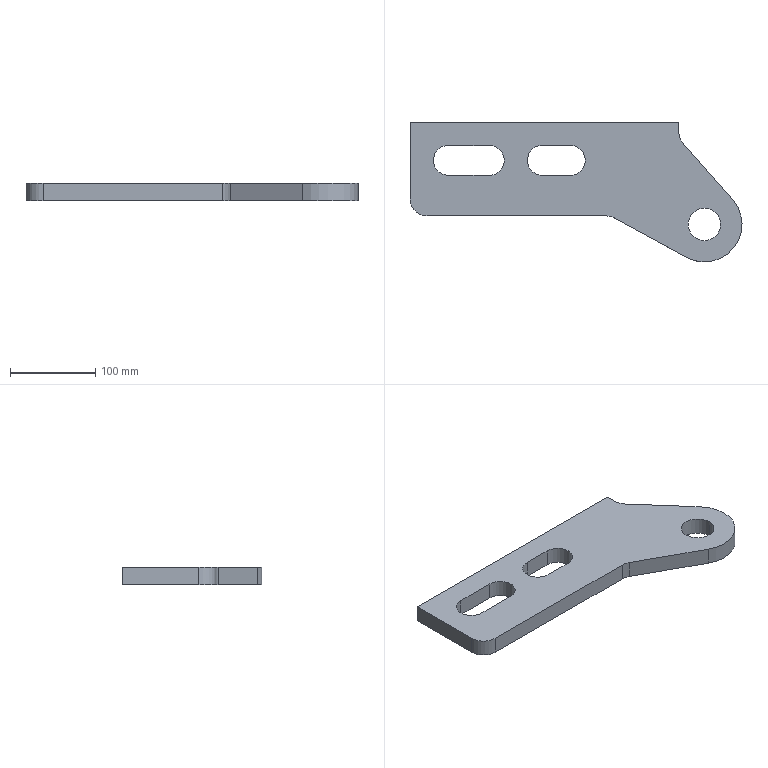Part | SolidWorks | features Extrusion 1 | 1 solid | 24 faces | box 389 x 164 x 20 mm | volume 749455 mm3 | cylinder 12 | plane 12 | commonest cylinder face diameters 35 x6 40 x3 38 x2 88 x1
STEP:
#1=CARTESIAN_POINT('',(-160.,-27.5,20.));
#2=VERTEX_POINT('',#1);
#3=CARTESIAN_POINT('',(-177.5,-45.,20.));
#4=VERTEX_POINT('',#3);
#5=CARTESIAN_POINT('',(-160.,-45.,20.));
#6=DIRECTION('',(0.,0.,1.));
#7=DIRECTION('',(1.,0.,0.));
#8=AXIS2_PLACEMENT_3D('',#5,#6,#7);
#9=CIRCLE('',#8,17.5);
#10=EDGE_CURVE('',#2,#4,#9,.T.);
#11=ORIENTED_EDGE('',*,*,#10,.T.);
#12=CARTESIAN_POINT('',(-177.5,-45.,0.));
#13=VERTEX_POINT('',#12);
#14=CARTESIAN_POINT('',(-177.5,-45.,20.));
#15=DIRECTION('',(0.,0.,-1.));
#16=VECTOR('',#15,1000.);
#17=LINE('',#14,#16);
#18=EDGE_CURVE('',#4,#13,#17,.T.);
#19=ORIENTED_EDGE('',*,*,#18,.T.);
#20=CARTESIAN_POINT('',(-160.,-27.5,0.));
#21=VERTEX_POINT('',#20);
#22=CARTESIAN_POINT('',(-160.,-45.,0.));
#23=DIRECTION('',(0.,0.,1.));
#24=DIRECTION('',(1.,0.,0.));
#25=AXIS2_PLACEMENT_3D('',#22,#23,#24);
#26=CIRCLE('',#25,17.5);
#27=EDGE_CURVE('',#21,#13,#26,.T.);
#28=ORIENTED_EDGE('',*,*,#27,.F.);
#29=CARTESIAN_POINT('',(-160.,-27.5,20.));
#30=DIRECTION('',(0.,0.,-1.));
#31=VECTOR('',#30,1000.);
#32=LINE('',#29,#31);
#33=EDGE_CURVE('',#2,#21,#32,.T.);
#34=ORIENTED_EDGE('',*,*,#33,.F.);
#35=EDGE_LOOP('',(#11,#19,#28,#34));
#36=FACE_OUTER_BOUND('',#35,.T.);
#37=CARTESIAN_POINT('',(-160.,-45.,20.));
#38=DIRECTION('',(0.,0.,-1.));
#39=DIRECTION('',(-1.,0.,0.));
#40=AXIS2_PLACEMENT_3D('',#37,#38,#39);
#41=CYLINDRICAL_SURFACE('',#40,17.5);
#42=ADVANCED_FACE('',(#36),#41,.F.);
#43=CARTESIAN_POINT('',(-270.,-27.5,20.));
#44=VERTEX_POINT('',#43);
#45=CARTESIAN_POINT('',(-287.5,-45.,20.));
#46=VERTEX_POINT('',#45);
#47=CARTESIAN_POINT('',(-270.,-45.,20.));
#48=DIRECTION('',(0.,0.,1.));
#49=DIRECTION('',(1.,0.,0.));
#50=AXIS2_PLACEMENT_3D('',#47,#48,#49);
#51=CIRCLE('',#50,17.5);
#52=EDGE_CURVE('',#44,#46,#51,.T.);
#53=ORIENTED_EDGE('',*,*,#52,.T.);
#54=CARTESIAN_POINT('',(-287.5,-45.,0.));
#55=VERTEX_POINT('',#54);
#56=CARTESIAN_POINT('',(-287.5,-45.,20.));
#57=DIRECTION('',(0.,0.,-1.));
#58=VECTOR('',#57,1000.);
#59=LINE('',#56,#58);
#60=EDGE_CURVE('',#46,#55,#59,.T.);
#61=ORIENTED_EDGE('',*,*,#60,.T.);
#62=CARTESIAN_POINT('',(-270.,-27.5,0.));
#63=VERTEX_POINT('',#62);
#64=CARTESIAN_POINT('',(-270.,-45.,0.));
#65=DIRECTION('',(0.,0.,1.));
#66=DIRECTION('',(1.,0.,0.));
#67=AXIS2_PLACEMENT_3D('',#64,#65,#66);
#68=CIRCLE('',#67,17.5);
#69=EDGE_CURVE('',#63,#55,#68,.T.);
#70=ORIENTED_EDGE('',*,*,#69,.F.);
#71=CARTESIAN_POINT('',(-270.,-27.5,20.));
#72=DIRECTION('',(0.,0.,-1.));
#73=VECTOR('',#72,1000.);
#74=LINE('',#71,#73);
#75=EDGE_CURVE('',#44,#63,#74,.T.);
#76=ORIENTED_EDGE('',*,*,#75,.F.);
#77=EDGE_LOOP('',(#53,#61,#70,#76));
#78=FACE_OUTER_BOUND('',#77,.T.);
#79=CARTESIAN_POINT('',(-270.,-45.,20.));
#80=DIRECTION('',(0.,0.,-1.));
#81=DIRECTION('',(-1.,0.,0.));
#82=AXIS2_PLACEMENT_3D('',#79,#80,#81);
#83=CYLINDRICAL_SURFACE('',#82,17.5);
#84=ADVANCED_FACE('',(#78),#83,.F.);
#85=CARTESIAN_POINT('',(11.,-120.,20.));
#86=VERTEX_POINT('',#85);
#87=CARTESIAN_POINT('',(49.,-120.,20.));
#88=VERTEX_POINT('',#87);
#89=CARTESIAN_POINT('',(30.,-120.,20.));
#90=DIRECTION('',(0.,0.,1.));
#91=DIRECTION('',(1.,0.,0.));
#92=AXIS2_PLACEMENT_3D('',#89,#90,#91);
#93=CIRCLE('',#92,19.);
#94=EDGE_CURVE('',#86,#88,#93,.T.);
#95=ORIENTED_EDGE('',*,*,#94,.T.);
#96=CARTESIAN_POINT('',(49.,-120.,0.));
#97=VERTEX_POINT('',#96);
#98=CARTESIAN_POINT('',(49.,-120.,20.));
#99=DIRECTION('',(0.,0.,-1.));
#100=VECTOR('',#99,1000.);
#101=LINE('',#98,#100);
#102=EDGE_CURVE('',#88,#97,#101,.T.);
#103=ORIENTED_EDGE('',*,*,#102,.T.);
#104=CARTESIAN_POINT('',(11.,-120.,0.));
#105=VERTEX_POINT('',#104);
#106=CARTESIAN_POINT('',(30.,-120.,0.));
#107=DIRECTION('',(0.,0.,1.));
#108=DIRECTION('',(1.,0.,0.));
#109=AXIS2_PLACEMENT_3D('',#106,#107,#108);
#110=CIRCLE('',#109,19.);
#111=EDGE_CURVE('',#105,#97,#110,.T.);
#112=ORIENTED_EDGE('',*,*,#111,.F.);
#113=CARTESIAN_POINT('',(11.,-120.,20.));
#114=DIRECTION('',(0.,0.,-1.));
#115=VECTOR('',#114,1000.);
#116=LINE('',#113,#115);
#117=EDGE_CURVE('',#86,#105,#116,.T.);
#118=ORIENTED_EDGE('',*,*,#117,.F.);
#119=EDGE_LOOP('',(#95,#103,#112,#118));
#120=FACE_OUTER_BOUND('',#119,.T.);
#121=CARTESIAN_POINT('',(30.,-120.,20.));
#122=DIRECTION('',(0.,0.,-1.));
#123=DIRECTION('',(-1.,0.,0.));
#124=AXIS2_PLACEMENT_3D('',#121,#122,#123);
#125=CYLINDRICAL_SURFACE('',#124,19.);
#126=ADVANCED_FACE('',(#120),#125,.F.);
#127=CARTESIAN_POINT('',(0.,-11.718,20.));
#128=VERTEX_POINT('',#127);
#129=CARTESIAN_POINT('',(0.,0.,20.));
#130=VERTEX_POINT('',#129);
#131=CARTESIAN_POINT('',(0.,0.,20.));
#132=DIRECTION('',(0.,1.,0.));
#133=VECTOR('',#132,1000.);
#134=LINE('',#131,#133);
#135=EDGE_CURVE('',#128,#130,#134,.T.);
#136=ORIENTED_EDGE('',*,*,#135,.T.);
#137=CARTESIAN_POINT('',(-315.,0.,20.));
#138=VERTEX_POINT('',#137);
#139=CARTESIAN_POINT('',(0.,0.,20.));
#140=DIRECTION('',(-1.,0.,0.));
#141=VECTOR('',#140,1000.);
#142=LINE('',#139,#141);
#143=EDGE_CURVE('',#130,#138,#142,.T.);
#144=ORIENTED_EDGE('',*,*,#143,.T.);
#145=CARTESIAN_POINT('',(-315.,-90.,20.));
#146=VERTEX_POINT('',#145);
#147=CARTESIAN_POINT('',(-315.,0.,20.));
#148=DIRECTION('',(0.,-1.,0.));
#149=VECTOR('',#148,1000.);
#150=LINE('',#147,#149);
#151=EDGE_CURVE('',#138,#146,#150,.T.);
#152=ORIENTED_EDGE('',*,*,#151,.T.);
#153=CARTESIAN_POINT('',(-295.,-110.,20.));
#154=VERTEX_POINT('',#153);
#155=CARTESIAN_POINT('',(-295.,-90.,20.));
#156=DIRECTION('',(0.,0.,1.));
#157=DIRECTION('',(1.,0.,0.));
#158=AXIS2_PLACEMENT_3D('',#155,#156,#157);
#159=CIRCLE('',#158,20.);
#160=EDGE_CURVE('',#146,#154,#159,.T.);
#161=ORIENTED_EDGE('',*,*,#160,.T.);
#162=CARTESIAN_POINT('',(-85.111,-110.,20.));
#163=VERTEX_POINT('',#162);
#164=CARTESIAN_POINT('',(-295.,-110.,20.));
#165=DIRECTION('',(1.,0.,0.));
#166=VECTOR('',#165,1000.);
#167=LINE('',#164,#166);
#168=EDGE_CURVE('',#154,#163,#167,.T.);
#169=ORIENTED_EDGE('',*,*,#168,.T.);
#170=CARTESIAN_POINT('',(-75.516,-112.452,20.));
#171=VERTEX_POINT('',#170);
#172=CARTESIAN_POINT('',(-85.111,-130.,20.));
#173=DIRECTION('',(0.,0.,-1.));
#174=DIRECTION('',(-1.,0.,0.));
#175=AXIS2_PLACEMENT_3D('',#172,#173,#174);
#176=CIRCLE('',#175,20.);
#177=EDGE_CURVE('',#163,#171,#176,.T.);
#178=ORIENTED_EDGE('',*,*,#177,.T.);
#179=CARTESIAN_POINT('',(8.89,-158.606,20.));
#180=VERTEX_POINT('',#179);
#181=CARTESIAN_POINT('',(-75.516,-112.452,20.));
#182=DIRECTION('',(0.8774,-0.4798,0.));
#183=VECTOR('',#182,1000.);
#184=LINE('',#181,#183);
#185=EDGE_CURVE('',#171,#180,#184,.T.);
#186=ORIENTED_EDGE('',*,*,#185,.T.);
#187=CARTESIAN_POINT('',(63.04,-90.943,20.));
#188=VERTEX_POINT('',#187);
#189=CARTESIAN_POINT('',(30.,-120.,20.));
#190=DIRECTION('',(0.,0.,1.));
#191=DIRECTION('',(1.,0.,0.));
#192=AXIS2_PLACEMENT_3D('',#189,#190,#191);
#193=CIRCLE('',#192,44.);
#194=EDGE_CURVE('',#180,#188,#193,.T.);
#195=ORIENTED_EDGE('',*,*,#194,.T.);
#196=CARTESIAN_POINT('',(4.982,-24.926,20.));
#197=VERTEX_POINT('',#196);
#198=CARTESIAN_POINT('',(4.982,-24.926,20.));
#199=DIRECTION('',(-0.6604,0.7509,0.));
#200=VECTOR('',#199,1000.);
#201=LINE('',#198,#200);
#202=EDGE_CURVE('',#188,#197,#201,.T.);
#203=ORIENTED_EDGE('',*,*,#202,.T.);
#204=CARTESIAN_POINT('',(20.,-11.718,20.));
#205=DIRECTION('',(0.,0.,-1.));
#206=DIRECTION('',(1.,0.,0.));
#207=AXIS2_PLACEMENT_3D('',#204,#205,#206);
#208=CIRCLE('',#207,20.);
#209=EDGE_CURVE('',#197,#128,#208,.T.);
#210=ORIENTED_EDGE('',*,*,#209,.T.);
#211=EDGE_LOOP('',(#136,#144,#152,#161,#169,#178,#186,#195,#203,#210));
#212=FACE_OUTER_BOUND('',#211,.T.);
#213=ORIENTED_EDGE('',*,*,#94,.F.);
#214=CARTESIAN_POINT('',(30.,-120.,20.));
#215=DIRECTION('',(0.,0.,1.));
#216=DIRECTION('',(1.,0.,0.));
#217=AXIS2_PLACEMENT_3D('',#214,#215,#216);
#218=CIRCLE('',#217,19.);
#219=EDGE_CURVE('',#88,#86,#218,.T.);
#220=ORIENTED_EDGE('',*,*,#219,.F.);
#221=EDGE_LOOP('',(#213,#220));
#222=FACE_BOUND('',#221,.T.);
#223=CARTESIAN_POINT('',(-270.,-62.5,20.));
#224=VERTEX_POINT('',#223);
#225=CARTESIAN_POINT('',(-222.,-62.5,20.));
#226=VERTEX_POINT('',#225);
#227=CARTESIAN_POINT('',(-270.,-62.5,20.));
#228=DIRECTION('',(1.,0.,0.));
#229=VECTOR('',#228,1000.);
#230=LINE('',#227,#229);
#231=EDGE_CURVE('',#224,#226,#230,.T.);
#232=ORIENTED_EDGE('',*,*,#231,.F.);
#233=CARTESIAN_POINT('',(-270.,-45.,20.));
#234=DIRECTION('',(0.,0.,1.));
#235=DIRECTION('',(1.,0.,0.));
#236=AXIS2_PLACEMENT_3D('',#233,#234,#235);
#237=CIRCLE('',#236,17.5);
#238=EDGE_CURVE('',#46,#224,#237,.T.);
#239=ORIENTED_EDGE('',*,*,#238,.F.);
#240=ORIENTED_EDGE('',*,*,#52,.F.);
#241=CARTESIAN_POINT('',(-222.,-27.5,20.));
#242=VERTEX_POINT('',#241);
#243=CARTESIAN_POINT('',(-270.,-27.5,20.));
#244=DIRECTION('',(-1.,0.,0.));
#245=VECTOR('',#244,1000.);
#246=LINE('',#243,#245);
#247=EDGE_CURVE('',#242,#44,#246,.T.);
#248=ORIENTED_EDGE('',*,*,#247,.F.);
#249=CARTESIAN_POINT('',(-222.,-45.,20.));
#250=DIRECTION('',(0.,0.,1.));
#251=DIRECTION('',(1.,0.,0.));
#252=AXIS2_PLACEMENT_3D('',#249,#250,#251);
#253=CIRCLE('',#252,17.5);
#254=EDGE_CURVE('',#226,#242,#253,.T.);
#255=ORIENTED_EDGE('',*,*,#254,.F.);
#256=EDGE_LOOP('',(#232,#239,#240,#248,#255));
#257=FACE_BOUND('',#256,.T.);
#258=CARTESIAN_POINT('',(-160.,-62.5,20.));
#259=VERTEX_POINT('',#258);
#260=CARTESIAN_POINT('',(-127.,-62.5,20.));
#261=VERTEX_POINT('',#260);
#262=CARTESIAN_POINT('',(-160.,-62.5,20.));
#263=DIRECTION('',(1.,0.,0.));
#264=VECTOR('',#263,1000.);
#265=LINE('',#262,#264);
#266=EDGE_CURVE('',#259,#261,#265,.T.);
#267=ORIENTED_EDGE('',*,*,#266,.F.);
#268=CARTESIAN_POINT('',(-160.,-45.,20.));
#269=DIRECTION('',(0.,0.,1.));
#270=DIRECTION('',(1.,0.,0.));
#271=AXIS2_PLACEMENT_3D('',#268,#269,#270);
#272=CIRCLE('',#271,17.5);
#273=EDGE_CURVE('',#4,#259,#272,.T.);
#274=ORIENTED_EDGE('',*,*,#273,.F.);
#275=ORIENTED_EDGE('',*,*,#10,.F.);
#276=CARTESIAN_POINT('',(-127.,-27.5,20.));
#277=VERTEX_POINT('',#276);
#278=CARTESIAN_POINT('',(-160.,-27.5,20.));
#279=DIRECTION('',(-1.,0.,0.));
#280=VECTOR('',#279,1000.);
#281=LINE('',#278,#280);
#282=EDGE_CURVE('',#277,#2,#281,.T.);
#283=ORIENTED_EDGE('',*,*,#282,.F.);
#284=CARTESIAN_POINT('',(-127.,-45.,20.));
#285=DIRECTION('',(0.,0.,1.));
#286=DIRECTION('',(1.,0.,0.));
#287=AXIS2_PLACEMENT_3D('',#284,#285,#286);
#288=CIRCLE('',#287,17.5);
#289=EDGE_CURVE('',#261,#277,#288,.T.);
#290=ORIENTED_EDGE('',*,*,#289,.F.);
#291=EDGE_LOOP('',(#267,#274,#275,#283,#290));
#292=FACE_BOUND('',#291,.T.);
#293=CARTESIAN_POINT('',(20.,-11.718,20.));
#294=DIRECTION('',(0.,0.,1.));
#295=DIRECTION('',(1.,0.,0.));
#296=AXIS2_PLACEMENT_3D('',#293,#294,#295);
#297=PLANE('',#296);
#298=ADVANCED_FACE('',(#212,#222,#257,#292),#297,.T.);
#299=ORIENTED_EDGE('',*,*,#69,.T.);
#300=CARTESIAN_POINT('',(-270.,-62.5,0.));
#301=VERTEX_POINT('',#300);
#302=CARTESIAN_POINT('',(-270.,-45.,0.));
#303=DIRECTION('',(0.,0.,1.));
#304=DIRECTION('',(1.,0.,0.));
#305=AXIS2_PLACEMENT_3D('',#302,#303,#304);
#306=CIRCLE('',#305,17.5);
#307=EDGE_CURVE('',#55,#301,#306,.T.);
#308=ORIENTED_EDGE('',*,*,#307,.T.);
#309=CARTESIAN_POINT('',(-222.,-62.5,0.));
#310=VERTEX_POINT('',#309);
#311=CARTESIAN_POINT('',(-270.,-62.5,0.));
#312=DIRECTION('',(1.,0.,0.));
#313=VECTOR('',#312,1000.);
#314=LINE('',#311,#313);
#315=EDGE_CURVE('',#301,#310,#314,.T.);
#316=ORIENTED_EDGE('',*,*,#315,.T.);
#317=CARTESIAN_POINT('',(-222.,-27.5,0.));
#318=VERTEX_POINT('',#317);
#319=CARTESIAN_POINT('',(-222.,-45.,0.));
#320=DIRECTION('',(0.,0.,1.));
#321=DIRECTION('',(1.,0.,0.));
#322=AXIS2_PLACEMENT_3D('',#319,#320,#321);
#323=CIRCLE('',#322,17.5);
#324=EDGE_CURVE('',#310,#318,#323,.T.);
#325=ORIENTED_EDGE('',*,*,#324,.T.);
#326=CARTESIAN_POINT('',(-270.,-27.5,0.));
#327=DIRECTION('',(-1.,0.,0.));
#328=VECTOR('',#327,1000.);
#329=LINE('',#326,#328);
#330=EDGE_CURVE('',#318,#63,#329,.T.);
#331=ORIENTED_EDGE('',*,*,#330,.T.);
#332=EDGE_LOOP('',(#299,#308,#316,#325,#331));
#333=FACE_BOUND('',#332,.T.);
#334=CARTESIAN_POINT('',(0.,-11.718,0.));
#335=VERTEX_POINT('',#334);
#336=CARTESIAN_POINT('',(0.,0.,0.));
#337=VERTEX_POINT('',#336);
#338=CARTESIAN_POINT('',(0.,0.,0.));
#339=DIRECTION('',(0.,1.,0.));
#340=VECTOR('',#339,1000.);
#341=LINE('',#338,#340);
#342=EDGE_CURVE('',#335,#337,#341,.T.);
#343=ORIENTED_EDGE('',*,*,#342,.F.);
#344=CARTESIAN_POINT('',(4.982,-24.926,0.));
#345=VERTEX_POINT('',#344);
#346=CARTESIAN_POINT('',(20.,-11.718,0.));
#347=DIRECTION('',(0.,0.,-1.));
#348=DIRECTION('',(1.,0.,0.));
#349=AXIS2_PLACEMENT_3D('',#346,#347,#348);
#350=CIRCLE('',#349,20.);
#351=EDGE_CURVE('',#345,#335,#350,.T.);
#352=ORIENTED_EDGE('',*,*,#351,.F.);
#353=CARTESIAN_POINT('',(63.04,-90.943,0.));
#354=VERTEX_POINT('',#353);
#355=CARTESIAN_POINT('',(4.982,-24.926,0.));
#356=DIRECTION('',(-0.6604,0.7509,0.));
#357=VECTOR('',#356,1000.);
#358=LINE('',#355,#357);
#359=EDGE_CURVE('',#354,#345,#358,.T.);
#360=ORIENTED_EDGE('',*,*,#359,.F.);
#361=CARTESIAN_POINT('',(8.89,-158.606,0.));
#362=VERTEX_POINT('',#361);
#363=CARTESIAN_POINT('',(30.,-120.,0.));
#364=DIRECTION('',(0.,0.,1.));
#365=DIRECTION('',(1.,0.,0.));
#366=AXIS2_PLACEMENT_3D('',#363,#364,#365);
#367=CIRCLE('',#366,44.);
#368=EDGE_CURVE('',#362,#354,#367,.T.);
#369=ORIENTED_EDGE('',*,*,#368,.F.);
#370=CARTESIAN_POINT('',(-75.516,-112.452,0.));
#371=VERTEX_POINT('',#370);
#372=CARTESIAN_POINT('',(-75.516,-112.452,0.));
#373=DIRECTION('',(0.8774,-0.4798,0.));
#374=VECTOR('',#373,1000.);
#375=LINE('',#372,#374);
#376=EDGE_CURVE('',#371,#362,#375,.T.);
#377=ORIENTED_EDGE('',*,*,#376,.F.);
#378=CARTESIAN_POINT('',(-85.111,-110.,0.));
#379=VERTEX_POINT('',#378);
#380=CARTESIAN_POINT('',(-85.111,-130.,0.));
#381=DIRECTION('',(0.,0.,-1.));
#382=DIRECTION('',(-1.,0.,0.));
#383=AXIS2_PLACEMENT_3D('',#380,#381,#382);
#384=CIRCLE('',#383,20.);
#385=EDGE_CURVE('',#379,#371,#384,.T.);
#386=ORIENTED_EDGE('',*,*,#385,.F.);
#387=CARTESIAN_POINT('',(-295.,-110.,0.));
#388=VERTEX_POINT('',#387);
#389=CARTESIAN_POINT('',(-295.,-110.,0.));
#390=DIRECTION('',(1.,0.,0.));
#391=VECTOR('',#390,1000.);
#392=LINE('',#389,#391);
#393=EDGE_CURVE('',#388,#379,#392,.T.);
#394=ORIENTED_EDGE('',*,*,#393,.F.);
#395=CARTESIAN_POINT('',(-315.,-90.,0.));
#396=VERTEX_POINT('',#395);
#397=CARTESIAN_POINT('',(-295.,-90.,0.));
#398=DIRECTION('',(0.,0.,1.));
#399=DIRECTION('',(1.,0.,0.));
#400=AXIS2_PLACEMENT_3D('',#397,#398,#399);
#401=CIRCLE('',#400,20.);
#402=EDGE_CURVE('',#396,#388,#401,.T.);
#403=ORIENTED_EDGE('',*,*,#402,.F.);
#404=CARTESIAN_POINT('',(-315.,0.,0.));
#405=VERTEX_POINT('',#404);
#406=CARTESIAN_POINT('',(-315.,0.,0.));
#407=DIRECTION('',(0.,-1.,0.));
#408=VECTOR('',#407,1000.);
#409=LINE('',#406,#408);
#410=EDGE_CURVE('',#405,#396,#409,.T.);
#411=ORIENTED_EDGE('',*,*,#410,.F.);
#412=CARTESIAN_POINT('',(0.,0.,0.));
#413=DIRECTION('',(-1.,0.,0.));
#414=VECTOR('',#413,1000.);
#415=LINE('',#412,#414);
#416=EDGE_CURVE('',#337,#405,#415,.T.);
#417=ORIENTED_EDGE('',*,*,#416,.F.);
#418=EDGE_LOOP('',(#343,#352,#360,#369,#377,#386,#394,#403,#411,#417));
#419=FACE_OUTER_BOUND('',#418,.T.);
#420=ORIENTED_EDGE('',*,*,#111,.T.);
#421=CARTESIAN_POINT('',(30.,-120.,0.));
#422=DIRECTION('',(0.,0.,1.));
#423=DIRECTION('',(1.,0.,0.));
#424=AXIS2_PLACEMENT_3D('',#421,#422,#423);
#425=CIRCLE('',#424,19.);
#426=EDGE_CURVE('',#97,#105,#425,.T.);
#427=ORIENTED_EDGE('',*,*,#426,.T.);
#428=EDGE_LOOP('',(#420,#427));
#429=FACE_BOUND('',#428,.T.);
#430=ORIENTED_EDGE('',*,*,#27,.T.);
#431=CARTESIAN_POINT('',(-160.,-62.5,0.));
#432=VERTEX_POINT('',#431);
#433=CARTESIAN_POINT('',(-160.,-45.,0.));
#434=DIRECTION('',(0.,0.,1.));
#435=DIRECTION('',(1.,0.,0.));
#436=AXIS2_PLACEMENT_3D('',#433,#434,#435);
#437=CIRCLE('',#436,17.5);
#438=EDGE_CURVE('',#13,#432,#437,.T.);
#439=ORIENTED_EDGE('',*,*,#438,.T.);
#440=CARTESIAN_POINT('',(-127.,-62.5,0.));
#441=VERTEX_POINT('',#440);
#442=CARTESIAN_POINT('',(-160.,-62.5,0.));
#443=DIRECTION('',(1.,0.,0.));
#444=VECTOR('',#443,1000.);
#445=LINE('',#442,#444);
#446=EDGE_CURVE('',#432,#441,#445,.T.);
#447=ORIENTED_EDGE('',*,*,#446,.T.);
#448=CARTESIAN_POINT('',(-127.,-27.5,0.));
#449=VERTEX_POINT('',#448);
#450=CARTESIAN_POINT('',(-127.,-45.,0.));
#451=DIRECTION('',(0.,0.,1.));
#452=DIRECTION('',(1.,0.,0.));
#453=AXIS2_PLACEMENT_3D('',#450,#451,#452);
#454=CIRCLE('',#453,17.5);
#455=EDGE_CURVE('',#441,#449,#454,.T.);
#456=ORIENTED_EDGE('',*,*,#455,.T.);
#457=CARTESIAN_POINT('',(-160.,-27.5,0.));
#458=DIRECTION('',(-1.,0.,0.));
#459=VECTOR('',#458,1000.);
#460=LINE('',#457,#459);
#461=EDGE_CURVE('',#449,#21,#460,.T.);
#462=ORIENTED_EDGE('',*,*,#461,.T.);
#463=EDGE_LOOP('',(#430,#439,#447,#456,#462));
#464=FACE_BOUND('',#463,.T.);
#465=CARTESIAN_POINT('',(20.,-11.718,0.));
#466=DIRECTION('',(0.,0.,1.));
#467=DIRECTION('',(1.,0.,0.));
#468=AXIS2_PLACEMENT_3D('',#465,#466,#467);
#469=PLANE('',#468);
#470=ADVANCED_FACE('',(#333,#419,#429,#464),#469,.F.);
#471=ORIENTED_EDGE('',*,*,#342,.T.);
#472=CARTESIAN_POINT('',(0.,0.,20.));
#473=DIRECTION('',(0.,0.,-1.));
#474=VECTOR('',#473,1000.);
#475=LINE('',#472,#474);
#476=EDGE_CURVE('',#130,#337,#475,.T.);
#477=ORIENTED_EDGE('',*,*,#476,.F.);
#478=ORIENTED_EDGE('',*,*,#135,.F.);
#479=CARTESIAN_POINT('',(0.,-11.718,20.));
#480=DIRECTION('',(0.,0.,-1.));
#481=VECTOR('',#480,1000.);
#482=LINE('',#479,#481);
#483=EDGE_CURVE('',#128,#335,#482,.T.);
#484=ORIENTED_EDGE('',*,*,#483,.T.);
#485=EDGE_LOOP('',(#471,#477,#478,#484));
#486=FACE_OUTER_BOUND('',#485,.T.);
#487=CARTESIAN_POINT('',(0.,0.,20.));
#488=DIRECTION('',(-1.,0.,0.));
#489=DIRECTION('',(0.,-1.,0.));
#490=AXIS2_PLACEMENT_3D('',#487,#488,#489);
#491=PLANE('',#490);
#492=ADVANCED_FACE('',(#486),#491,.F.);
#493=ORIENTED_EDGE('',*,*,#416,.T.);
#494=CARTESIAN_POINT('',(-315.,0.,20.));
#495=DIRECTION('',(0.,0.,-1.));
#496=VECTOR('',#495,1000.);
#497=LINE('',#494,#496);
#498=EDGE_CURVE('',#138,#405,#497,.T.);
#499=ORIENTED_EDGE('',*,*,#498,.F.);
#500=ORIENTED_EDGE('',*,*,#143,.F.);
#501=ORIENTED_EDGE('',*,*,#476,.T.);
#502=EDGE_LOOP('',(#493,#499,#500,#501));
#503=FACE_OUTER_BOUND('',#502,.T.);
#504=CARTESIAN_POINT('',(0.,0.,20.));
#505=DIRECTION('',(0.,-1.,0.));
#506=DIRECTION('',(1.,0.,0.));
#507=AXIS2_PLACEMENT_3D('',#504,#505,#506);
#508=PLANE('',#507);
#509=ADVANCED_FACE('',(#503),#508,.F.);
#510=ORIENTED_EDGE('',*,*,#410,.T.);
#511=CARTESIAN_POINT('',(-315.,-90.,20.));
#512=DIRECTION('',(0.,0.,-1.));
#513=VECTOR('',#512,1000.);
#514=LINE('',#511,#513);
#515=EDGE_CURVE('',#146,#396,#514,.T.);
#516=ORIENTED_EDGE('',*,*,#515,.F.);
#517=ORIENTED_EDGE('',*,*,#151,.F.);
#518=ORIENTED_EDGE('',*,*,#498,.T.);
#519=EDGE_LOOP('',(#510,#516,#517,#518));
#520=FACE_OUTER_BOUND('',#519,.T.);
#521=CARTESIAN_POINT('',(-315.,0.,20.));
#522=DIRECTION('',(1.,0.,0.));
#523=DIRECTION('',(0.,0.,-1.));
#524=AXIS2_PLACEMENT_3D('',#521,#522,#523);
#525=PLANE('',#524);
#526=ADVANCED_FACE('',(#520),#525,.F.);
#527=ORIENTED_EDGE('',*,*,#402,.T.);
#528=CARTESIAN_POINT('',(-295.,-110.,20.));
#529=DIRECTION('',(0.,0.,-1.));
#530=VECTOR('',#529,1000.);
#531=LINE('',#528,#530);
#532=EDGE_CURVE('',#154,#388,#531,.T.);
#533=ORIENTED_EDGE('',*,*,#532,.F.);
#534=ORIENTED_EDGE('',*,*,#160,.F.);
#535=ORIENTED_EDGE('',*,*,#515,.T.);
#536=EDGE_LOOP('',(#527,#533,#534,#535));
#537=FACE_OUTER_BOUND('',#536,.T.);
#538=CARTESIAN_POINT('',(-295.,-90.,20.));
#539=DIRECTION('',(0.,0.,-1.));
#540=DIRECTION('',(-1.,0.,0.));
#541=AXIS2_PLACEMENT_3D('',#538,#539,#540);
#542=CYLINDRICAL_SURFACE('',#541,20.);
#543=ADVANCED_FACE('',(#537),#542,.T.);
#544=ORIENTED_EDGE('',*,*,#393,.T.);
#545=CARTESIAN_POINT('',(-85.111,-110.,20.));
#546=DIRECTION('',(0.,0.,-1.));
#547=VECTOR('',#546,1000.);
#548=LINE('',#545,#547);
#549=EDGE_CURVE('',#163,#379,#548,.T.);
#550=ORIENTED_EDGE('',*,*,#549,.F.);
#551=ORIENTED_EDGE('',*,*,#168,.F.);
#552=ORIENTED_EDGE('',*,*,#532,.T.);
#553=EDGE_LOOP('',(#544,#550,#551,#552));
#554=FACE_OUTER_BOUND('',#553,.T.);
#555=CARTESIAN_POINT('',(-295.,-110.,20.));
#556=DIRECTION('',(0.,1.,0.));
#557=DIRECTION('',(0.,0.,1.));
#558=AXIS2_PLACEMENT_3D('',#555,#556,#557);
#559=PLANE('',#558);
#560=ADVANCED_FACE('',(#554),#559,.F.);
#561=ORIENTED_EDGE('',*,*,#385,.T.);
#562=CARTESIAN_POINT('',(-75.516,-112.452,20.));
#563=DIRECTION('',(0.,0.,-1.));
#564=VECTOR('',#563,1000.);
#565=LINE('',#562,#564);
#566=EDGE_CURVE('',#171,#371,#565,.T.);
#567=ORIENTED_EDGE('',*,*,#566,.F.);
#568=ORIENTED_EDGE('',*,*,#177,.F.);
#569=ORIENTED_EDGE('',*,*,#549,.T.);
#570=EDGE_LOOP('',(#561,#567,#568,#569));
#571=FACE_OUTER_BOUND('',#570,.T.);
#572=CARTESIAN_POINT('',(-85.111,-130.,20.));
#573=DIRECTION('',(0.,0.,-1.));
#574=DIRECTION('',(-1.,0.,0.));
#575=AXIS2_PLACEMENT_3D('',#572,#573,#574);
#576=CYLINDRICAL_SURFACE('',#575,20.);
#577=ADVANCED_FACE('',(#571),#576,.F.);
#578=ORIENTED_EDGE('',*,*,#376,.T.);
#579=CARTESIAN_POINT('',(8.89,-158.606,20.));
#580=DIRECTION('',(0.,0.,-1.));
#581=VECTOR('',#580,1000.);
#582=LINE('',#579,#581);
#583=EDGE_CURVE('',#180,#362,#582,.T.);
#584=ORIENTED_EDGE('',*,*,#583,.F.);
#585=ORIENTED_EDGE('',*,*,#185,.F.);
#586=ORIENTED_EDGE('',*,*,#566,.T.);
#587=EDGE_LOOP('',(#578,#584,#585,#586));
#588=FACE_OUTER_BOUND('',#587,.T.);
#589=CARTESIAN_POINT('',(-75.516,-112.452,20.));
#590=DIRECTION('',(0.4798,0.8774,0.));
#591=DIRECTION('',(-0.8774,0.4798,0.));
#592=AXIS2_PLACEMENT_3D('',#589,#590,#591);
#593=PLANE('',#592);
#594=ADVANCED_FACE('',(#588),#593,.F.);
#595=ORIENTED_EDGE('',*,*,#368,.T.);
#596=CARTESIAN_POINT('',(63.04,-90.943,20.));
#597=DIRECTION('',(0.,0.,-1.));
#598=VECTOR('',#597,1000.);
#599=LINE('',#596,#598);
#600=EDGE_CURVE('',#188,#354,#599,.T.);
#601=ORIENTED_EDGE('',*,*,#600,.F.);
#602=ORIENTED_EDGE('',*,*,#194,.F.);
#603=ORIENTED_EDGE('',*,*,#583,.T.);
#604=EDGE_LOOP('',(#595,#601,#602,#603));
#605=FACE_OUTER_BOUND('',#604,.T.);
#606=CARTESIAN_POINT('',(30.,-120.,20.));
#607=DIRECTION('',(0.,0.,-1.));
#608=DIRECTION('',(-1.,0.,0.));
#609=AXIS2_PLACEMENT_3D('',#606,#607,#608);
#610=CYLINDRICAL_SURFACE('',#609,44.);
#611=ADVANCED_FACE('',(#605),#610,.T.);
#612=ORIENTED_EDGE('',*,*,#359,.T.);
#613=CARTESIAN_POINT('',(4.982,-24.926,20.));
#614=DIRECTION('',(0.,0.,-1.));
#615=VECTOR('',#614,1000.);
#616=LINE('',#613,#615);
#617=EDGE_CURVE('',#197,#345,#616,.T.);
#618=ORIENTED_EDGE('',*,*,#617,.F.);
#619=ORIENTED_EDGE('',*,*,#202,.F.);
#620=ORIENTED_EDGE('',*,*,#600,.T.);
#621=EDGE_LOOP('',(#612,#618,#619,#620));
#622=FACE_OUTER_BOUND('',#621,.T.);
#623=CARTESIAN_POINT('',(4.982,-24.926,20.));
#624=DIRECTION('',(-0.7509,-0.6604,0.));
#625=DIRECTION('',(0.6604,-0.7509,0.));
#626=AXIS2_PLACEMENT_3D('',#623,#624,#625);
#627=PLANE('',#626);
#628=ADVANCED_FACE('',(#622),#627,.F.);
#629=ORIENTED_EDGE('',*,*,#351,.T.);
#630=ORIENTED_EDGE('',*,*,#483,.F.);
#631=ORIENTED_EDGE('',*,*,#209,.F.);
#632=ORIENTED_EDGE('',*,*,#617,.T.);
#633=EDGE_LOOP('',(#629,#630,#631,#632));
#634=FACE_OUTER_BOUND('',#633,.T.);
#635=CARTESIAN_POINT('',(20.,-11.718,20.));
#636=DIRECTION('',(0.,0.,-1.));
#637=DIRECTION('',(-1.,0.,0.));
#638=AXIS2_PLACEMENT_3D('',#635,#636,#637);
#639=CYLINDRICAL_SURFACE('',#638,20.);
#640=ADVANCED_FACE('',(#634),#639,.F.);
#641=ORIENTED_EDGE('',*,*,#102,.F.);
#642=ORIENTED_EDGE('',*,*,#219,.T.);
#643=ORIENTED_EDGE('',*,*,#117,.T.);
#644=ORIENTED_EDGE('',*,*,#426,.F.);
#645=EDGE_LOOP('',(#641,#642,#643,#644));
#646=FACE_OUTER_BOUND('',#645,.T.);
#647=CARTESIAN_POINT('',(30.,-120.,20.));
#648=DIRECTION('',(0.,0.,-1.));
#649=DIRECTION('',(-1.,0.,0.));
#650=AXIS2_PLACEMENT_3D('',#647,#648,#649);
#651=CYLINDRICAL_SURFACE('',#650,19.);
#652=ADVANCED_FACE('',(#646),#651,.F.);
#653=ORIENTED_EDGE('',*,*,#60,.F.);
#654=ORIENTED_EDGE('',*,*,#238,.T.);
#655=CARTESIAN_POINT('',(-270.,-62.5,20.));
#656=DIRECTION('',(0.,0.,-1.));
#657=VECTOR('',#656,1000.);
#658=LINE('',#655,#657);
#659=EDGE_CURVE('',#224,#301,#658,.T.);
#660=ORIENTED_EDGE('',*,*,#659,.T.);
#661=ORIENTED_EDGE('',*,*,#307,.F.);
#662=EDGE_LOOP('',(#653,#654,#660,#661));
#663=FACE_OUTER_BOUND('',#662,.T.);
#664=CARTESIAN_POINT('',(-270.,-45.,20.));
#665=DIRECTION('',(0.,0.,-1.));
#666=DIRECTION('',(-1.,0.,0.));
#667=AXIS2_PLACEMENT_3D('',#664,#665,#666);
#668=CYLINDRICAL_SURFACE('',#667,17.5);
#669=ADVANCED_FACE('',(#663),#668,.F.);
#670=ORIENTED_EDGE('',*,*,#315,.F.);
#671=ORIENTED_EDGE('',*,*,#659,.F.);
#672=ORIENTED_EDGE('',*,*,#231,.T.);
#673=CARTESIAN_POINT('',(-222.,-62.5,20.));
#674=DIRECTION('',(0.,0.,-1.));
#675=VECTOR('',#674,1000.);
#676=LINE('',#673,#675);
#677=EDGE_CURVE('',#226,#310,#676,.T.);
#678=ORIENTED_EDGE('',*,*,#677,.T.);
#679=EDGE_LOOP('',(#670,#671,#672,#678));
#680=FACE_OUTER_BOUND('',#679,.T.);
#681=CARTESIAN_POINT('',(-270.,-62.5,20.));
#682=DIRECTION('',(0.,1.,0.));
#683=DIRECTION('',(0.,0.,1.));
#684=AXIS2_PLACEMENT_3D('',#681,#682,#683);
#685=PLANE('',#684);
#686=ADVANCED_FACE('',(#680),#685,.T.);
#687=ORIENTED_EDGE('',*,*,#324,.F.);
#688=ORIENTED_EDGE('',*,*,#677,.F.);
#689=ORIENTED_EDGE('',*,*,#254,.T.);
#690=CARTESIAN_POINT('',(-222.,-27.5,20.));
#691=DIRECTION('',(0.,0.,-1.));
#692=VECTOR('',#691,1000.);
#693=LINE('',#690,#692);
#694=EDGE_CURVE('',#242,#318,#693,.T.);
#695=ORIENTED_EDGE('',*,*,#694,.T.);
#696=EDGE_LOOP('',(#687,#688,#689,#695));
#697=FACE_OUTER_BOUND('',#696,.T.);
#698=CARTESIAN_POINT('',(-222.,-45.,20.));
#699=DIRECTION('',(0.,0.,-1.));
#700=DIRECTION('',(-1.,0.,0.));
#701=AXIS2_PLACEMENT_3D('',#698,#699,#700);
#702=CYLINDRICAL_SURFACE('',#701,17.5);
#703=ADVANCED_FACE('',(#697),#702,.F.);
#704=ORIENTED_EDGE('',*,*,#330,.F.);
#705=ORIENTED_EDGE('',*,*,#694,.F.);
#706=ORIENTED_EDGE('',*,*,#247,.T.);
#707=ORIENTED_EDGE('',*,*,#75,.T.);
#708=EDGE_LOOP('',(#704,#705,#706,#707));
#709=FACE_OUTER_BOUND('',#708,.T.);
#710=CARTESIAN_POINT('',(-270.,-27.5,20.));
#711=DIRECTION('',(0.,-1.,0.));
#712=DIRECTION('',(1.,0.,0.));
#713=AXIS2_PLACEMENT_3D('',#710,#711,#712);
#714=PLANE('',#713);
#715=ADVANCED_FACE('',(#709),#714,.T.);
#716=ORIENTED_EDGE('',*,*,#18,.F.);
#717=ORIENTED_EDGE('',*,*,#273,.T.);
#718=CARTESIAN_POINT('',(-160.,-62.5,20.));
#719=DIRECTION('',(0.,0.,-1.));
#720=VECTOR('',#719,1000.);
#721=LINE('',#718,#720);
#722=EDGE_CURVE('',#259,#432,#721,.T.);
#723=ORIENTED_EDGE('',*,*,#722,.T.);
#724=ORIENTED_EDGE('',*,*,#438,.F.);
#725=EDGE_LOOP('',(#716,#717,#723,#724));
#726=FACE_OUTER_BOUND('',#725,.T.);
#727=CARTESIAN_POINT('',(-160.,-45.,20.));
#728=DIRECTION('',(0.,0.,-1.));
#729=DIRECTION('',(-1.,0.,0.));
#730=AXIS2_PLACEMENT_3D('',#727,#728,#729);
#731=CYLINDRICAL_SURFACE('',#730,17.5);
#732=ADVANCED_FACE('',(#726),#731,.F.);
#733=ORIENTED_EDGE('',*,*,#446,.F.);
#734=ORIENTED_EDGE('',*,*,#722,.F.);
#735=ORIENTED_EDGE('',*,*,#266,.T.);
#736=CARTESIAN_POINT('',(-127.,-62.5,20.));
#737=DIRECTION('',(0.,0.,-1.));
#738=VECTOR('',#737,1000.);
#739=LINE('',#736,#738);
#740=EDGE_CURVE('',#261,#441,#739,.T.);
#741=ORIENTED_EDGE('',*,*,#740,.T.);
#742=EDGE_LOOP('',(#733,#734,#735,#741));
#743=FACE_OUTER_BOUND('',#742,.T.);
#744=CARTESIAN_POINT('',(-160.,-62.5,20.));
#745=DIRECTION('',(0.,1.,0.));
#746=DIRECTION('',(0.,0.,1.));
#747=AXIS2_PLACEMENT_3D('',#744,#745,#746);
#748=PLANE('',#747);
#749=ADVANCED_FACE('',(#743),#748,.T.);
#750=ORIENTED_EDGE('',*,*,#455,.F.);
#751=ORIENTED_EDGE('',*,*,#740,.F.);
#752=ORIENTED_EDGE('',*,*,#289,.T.);
#753=CARTESIAN_POINT('',(-127.,-27.5,20.));
#754=DIRECTION('',(0.,0.,-1.));
#755=VECTOR('',#754,1000.);
#756=LINE('',#753,#755);
#757=EDGE_CURVE('',#277,#449,#756,.T.);
#758=ORIENTED_EDGE('',*,*,#757,.T.);
#759=EDGE_LOOP('',(#750,#751,#752,#758));
#760=FACE_OUTER_BOUND('',#759,.T.);
#761=CARTESIAN_POINT('',(-127.,-45.,20.));
#762=DIRECTION('',(0.,0.,-1.));
#763=DIRECTION('',(-1.,0.,0.));
#764=AXIS2_PLACEMENT_3D('',#761,#762,#763);
#765=CYLINDRICAL_SURFACE('',#764,17.5);
#766=ADVANCED_FACE('',(#760),#765,.F.);
#767=ORIENTED_EDGE('',*,*,#461,.F.);
#768=ORIENTED_EDGE('',*,*,#757,.F.);
#769=ORIENTED_EDGE('',*,*,#282,.T.);
#770=ORIENTED_EDGE('',*,*,#33,.T.);
#771=EDGE_LOOP('',(#767,#768,#769,#770));
#772=FACE_OUTER_BOUND('',#771,.T.);
#773=CARTESIAN_POINT('',(-160.,-27.5,20.));
#774=DIRECTION('',(0.,-1.,0.));
#775=DIRECTION('',(1.,0.,0.));
#776=AXIS2_PLACEMENT_3D('',#773,#774,#775);
#777=PLANE('',#776);
#778=ADVANCED_FACE('',(#772),#777,.T.);
#779=CLOSED_SHELL('',(#42,#84,#126,#298,#470,#492,#509,#526,#543,#560,#577,#594,#611,#628,#640,#652,#669,#686,#703,#715,#732,#749,#766,#778));
#780=MANIFOLD_SOLID_BREP('',#779);
#781=CARTESIAN_POINT('',(0.,0.,0.));
#782=DIRECTION('',(0.,0.,1.));
#783=DIRECTION('',(1.,0.,0.));
#784=AXIS2_PLACEMENT_3D('',#781,#782,#783);
#785=(LENGTH_UNIT()NAMED_UNIT(*)SI_UNIT(.MILLI.,.METRE.));
#786=UNCERTAINTY_MEASURE_WITH_UNIT(LENGTH_MEASURE(0.00001),#785,'','');
#787=(NAMED_UNIT(*)PLANE_ANGLE_UNIT()SI_UNIT($,.RADIAN.));
#788=(NAMED_UNIT(*)SI_UNIT($,.STERADIAN.)SOLID_ANGLE_UNIT());
#789=(GEOMETRIC_REPRESENTATION_CONTEXT(3)GLOBAL_UNCERTAINTY_ASSIGNED_CONTEXT((#786))GLOBAL_UNIT_ASSIGNED_CONTEXT((#785,#787,#788))REPRESENTATION_CONTEXT('',''));
#790=ADVANCED_BREP_SHAPE_REPRESENTATION('',(#780,#784),#789);